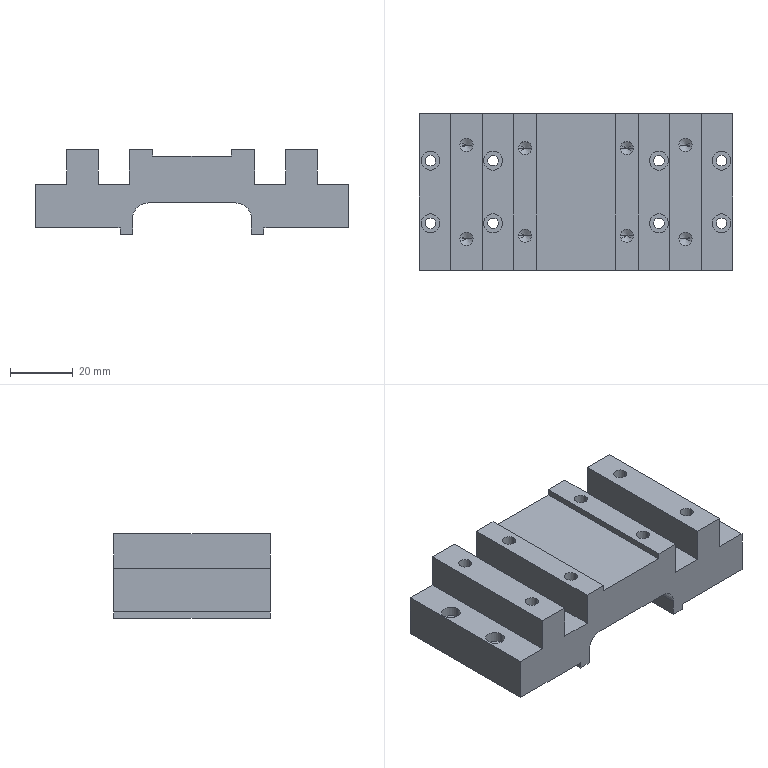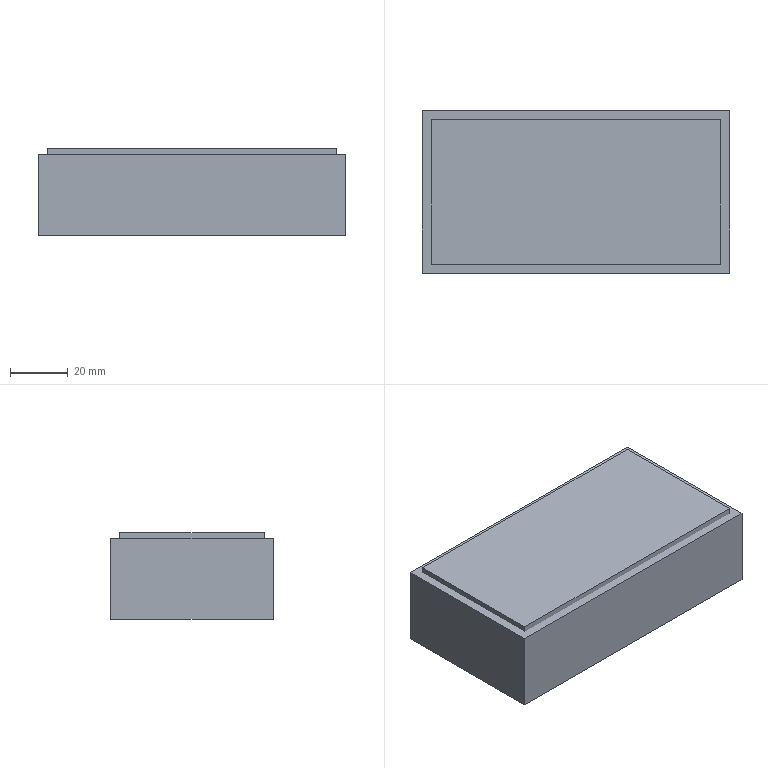CAM job | NX | 3-axis milling, drilling | part box 100 x 50 x 27 mm | stock box 106 x 56 x 30 mm
Tools:
number,name,description,diameter,corner_radius,flute_length,length,flutes
1,D50,Milling Tool-5 Parameters,50.0,0.0,50.0,75.0,2
2,D6A45,Milling Tool-5 Parameters,6.0,0.0,3.0,3.0,2
3,D10,Milling Tool-5 Parameters,10.0,0.0,50.0,75.0,2
4,D10JING,Milling Tool-5 Parameters,10.0,0.0,50.0,75.0,2
8,D6,Milling Tool-5 Parameters,6.0,0.0,50.0,75.0,2
14,4.2ZT,Drilling Tool,4.2,0.0,35.0,50.0,2
13,3.4ZT,Drilling Tool,3.4,0.0,35.0,50.0,2
10,D4,Milling Tool-5 Parameters,4.0,0.0,50.0,75.0,2
11,D6R0.5,Milling Tool-5 Parameters,6.0,0.5,50.0,75.0,2
Operations:
program,operation,operation_type,tool,method,geometry_group,spindle_rpm,surface_speed,feed_per_tooth,feed_cut,feed_plunge,cut_length_mm,path_length_mm,cut_time_min,machine_time_min
1-103-50-30毛胚,FLOOR_WALL,VolumeBased25DMillingOperation,D50,METHOD,A,6500.0,1286.0,0.0962,1250.0,100.0,359.997,413.997,0.288,0.2934
1-103-50-30毛胚,ADAPTIVE_MILLING,CavityMilling,D10,METHOD,A,7000.0,219.0,0.2143,3000.0,1000.0,9857.388,10889.558,3.304,3.407
1-103-50-30毛胚,ZLEVEL_PROFILE_COPY_COPY_1_COPY_COPY_COPY_1,ZLevelMilling,D10JING,METHOD,A,7000.0,219.0,0.0714,1000.0,100.0,669.097,783.284,0.6691,0.6805
1-103-50-30毛胚,FLOOR_WALL_1_COPY_1,VolumeBased25DMillingOperation,D10JING,METHOD,A,7000.0,87.0,0.0714,1000.0,100.0,934.534,1452.365,0.9345,0.9948
1-103-50-30毛胚,ZLEVEL_PROFILE_COPY_COPY_1_COPY_COPY_COPY_1_COPY,ZLevelMilling,D6,METHOD,A,7000.0,131.0,0.1786,2500.0,100.0,5117.473,5638.925,2.047,2.099
1-103-50-30毛胚,ZLEVEL_PROFILE_COPY_COPY_1_COPY_COPY_COPY_1_COPY_1,ZLevelMilling,D6,METHOD,A,7000.0,219.0,0.0714,1000.0,100.0,232.445,613.308,0.2324,0.2705
1-103-50-30毛胚,DRILLING_COPY_1,Operation,D6A45,METHOD,A,3000.0,56.0,0.0333,200.0,0.0,64.0,522.686,0.32,0.3659
1-103-50-30毛胚,DRILLING_COPY_1_COPY_COPY_COPY_COPY_1,Operation,4.2ZT,METHOD,A,2000.0,20.0,0.0375,150.0,0.0,146.095,542.186,0.974,1.014
1-103-50-30毛胚,DRILLING_COPY_1_COPY_COPY_COPY_COPY,Operation,3.4ZT,METHOD,A,2000.0,20.0,0.0375,150.0,0.0,148.172,573.771,0.9878,1.03
1-103-50-30毛胚,HOLE_MILLING,CylinderMilling,D4,METHOD,A,7000.0,131.0,0.1071,1500.0,100.0,729.594,1581.794,0.4864,0.5716
1-103-50-30毛胚,ZLEVEL_PROFILE_COPY_1_COPY_COPY_COPY_COPY_2_COPY,ZLevelMilling,D6A45,METHOD,A,7000.0,131.0,0.0714,1000.0,1000.0,990.632,3925.936,0.9906,1.284
2-103-50-30毛胚,FLOOR_WALL_COPY,VolumeBased25DMillingOperation,D50,METHOD,B,6500.0,1286.0,0.0962,1250.0,100.0,1025.991,1241.986,0.8208,0.8424
2-103-50-30毛胚,ADAPTIVE_MILLING_COPY,CavityMilling,D10,METHOD,B,7000.0,219.0,0.2143,3000.0,1000.0,12764.902,14047.479,4.281,4.409
2-103-50-30毛胚,FLOOR_WALL_1_COPY_1_COPY,VolumeBased25DMillingOperation,D10JING,METHOD,B,7000.0,87.0,0.0714,1000.0,100.0,1503.07,1996.687,1.503,1.563
2-103-50-30毛胚,ZLEVEL_PROFILE_COPY_COPY_1_COPY_COPY_COPY_1_COPY_2,ZLevelMilling,D10JING,METHOD,B,7000.0,219.0,0.0714,1000.0,100.0,127.306,293.435,0.1273,0.1439
2-103-50-30毛胚,ZLEVEL_PROFILE_COPY_COPY_1_COPY_COPY_COPY_1_COPY_1_COPY,ZLevelMilling,D6R0.5,METHOD,B,7000.0,131.0,0.2143,3000.0,1000.0,8848.443,9062.245,2.951,2.972
2-103-50-30毛胚,ZLEVEL_PROFILE_COPY_1_COPY_COPY_COPY_COPY_2_COPY_COPY,ZLevelMilling,D6A45,METHOD,B,7000.0,131.0,0.0714,1000.0,1000.0,616.505,1859.934,0.6165,0.7408